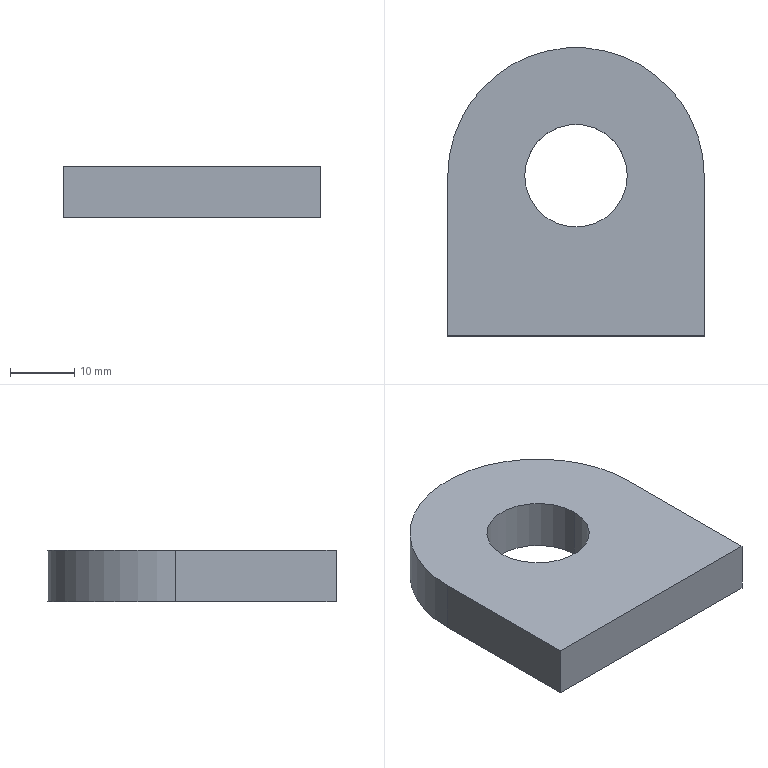Part | SolidWorks | features Extrusion 1 | 1 solid | 8 faces | box 40 x 45 x 8 mm | volume 11418 mm3 | plane 5 | cylinder 3 | commonest cylinder face diameters 16 x2 40 x1
STEP:
#1=CARTESIAN_POINT('',(-8.,0.,8.));
#2=VERTEX_POINT('',#1);
#3=CARTESIAN_POINT('',(8.,0.,8.));
#4=VERTEX_POINT('',#3);
#5=CARTESIAN_POINT('',(0.,0.,8.));
#6=DIRECTION('',(0.,0.,1.));
#7=DIRECTION('',(1.,0.,0.));
#8=AXIS2_PLACEMENT_3D('',#5,#6,#7);
#9=CIRCLE('',#8,8.);
#10=EDGE_CURVE('',#2,#4,#9,.T.);
#11=ORIENTED_EDGE('',*,*,#10,.T.);
#12=CARTESIAN_POINT('',(8.,0.,0.));
#13=VERTEX_POINT('',#12);
#14=CARTESIAN_POINT('',(8.,0.,8.));
#15=DIRECTION('',(0.,0.,-1.));
#16=VECTOR('',#15,1000.);
#17=LINE('',#14,#16);
#18=EDGE_CURVE('',#4,#13,#17,.T.);
#19=ORIENTED_EDGE('',*,*,#18,.T.);
#20=CARTESIAN_POINT('',(-8.,0.,0.));
#21=VERTEX_POINT('',#20);
#22=CARTESIAN_POINT('',(0.,0.,0.));
#23=DIRECTION('',(0.,0.,1.));
#24=DIRECTION('',(1.,0.,0.));
#25=AXIS2_PLACEMENT_3D('',#22,#23,#24);
#26=CIRCLE('',#25,8.);
#27=EDGE_CURVE('',#21,#13,#26,.T.);
#28=ORIENTED_EDGE('',*,*,#27,.F.);
#29=CARTESIAN_POINT('',(-8.,0.,8.));
#30=DIRECTION('',(0.,0.,-1.));
#31=VECTOR('',#30,1000.);
#32=LINE('',#29,#31);
#33=EDGE_CURVE('',#2,#21,#32,.T.);
#34=ORIENTED_EDGE('',*,*,#33,.F.);
#35=EDGE_LOOP('',(#11,#19,#28,#34));
#36=FACE_OUTER_BOUND('',#35,.T.);
#37=CARTESIAN_POINT('',(0.,0.,8.));
#38=DIRECTION('',(0.,0.,-1.));
#39=DIRECTION('',(-1.,0.,0.));
#40=AXIS2_PLACEMENT_3D('',#37,#38,#39);
#41=CYLINDRICAL_SURFACE('',#40,8.);
#42=ADVANCED_FACE('',(#36),#41,.F.);
#43=CARTESIAN_POINT('',(20.,-25.,8.));
#44=VERTEX_POINT('',#43);
#45=CARTESIAN_POINT('',(20.,0.,8.));
#46=VERTEX_POINT('',#45);
#47=CARTESIAN_POINT('',(20.,-25.,8.));
#48=DIRECTION('',(0.,1.,0.));
#49=VECTOR('',#48,1000.);
#50=LINE('',#47,#49);
#51=EDGE_CURVE('',#44,#46,#50,.T.);
#52=ORIENTED_EDGE('',*,*,#51,.T.);
#53=CARTESIAN_POINT('',(-20.,0.,8.));
#54=VERTEX_POINT('',#53);
#55=CARTESIAN_POINT('',(0.,0.,8.));
#56=DIRECTION('',(0.,0.,1.));
#57=DIRECTION('',(1.,0.,0.));
#58=AXIS2_PLACEMENT_3D('',#55,#56,#57);
#59=CIRCLE('',#58,20.);
#60=EDGE_CURVE('',#46,#54,#59,.T.);
#61=ORIENTED_EDGE('',*,*,#60,.T.);
#62=CARTESIAN_POINT('',(-20.,-25.,8.));
#63=VERTEX_POINT('',#62);
#64=CARTESIAN_POINT('',(-20.,0.,8.));
#65=DIRECTION('',(0.,-1.,0.));
#66=VECTOR('',#65,1000.);
#67=LINE('',#64,#66);
#68=EDGE_CURVE('',#54,#63,#67,.T.);
#69=ORIENTED_EDGE('',*,*,#68,.T.);
#70=CARTESIAN_POINT('',(-20.,-25.,8.));
#71=DIRECTION('',(1.,0.,0.));
#72=VECTOR('',#71,1000.);
#73=LINE('',#70,#72);
#74=EDGE_CURVE('',#63,#44,#73,.T.);
#75=ORIENTED_EDGE('',*,*,#74,.T.);
#76=EDGE_LOOP('',(#52,#61,#69,#75));
#77=FACE_OUTER_BOUND('',#76,.T.);
#78=ORIENTED_EDGE('',*,*,#10,.F.);
#79=CARTESIAN_POINT('',(0.,0.,8.));
#80=DIRECTION('',(0.,0.,1.));
#81=DIRECTION('',(1.,0.,0.));
#82=AXIS2_PLACEMENT_3D('',#79,#80,#81);
#83=CIRCLE('',#82,8.);
#84=EDGE_CURVE('',#4,#2,#83,.T.);
#85=ORIENTED_EDGE('',*,*,#84,.F.);
#86=EDGE_LOOP('',(#78,#85));
#87=FACE_BOUND('',#86,.T.);
#88=CARTESIAN_POINT('',(0.,0.,8.));
#89=DIRECTION('',(0.,0.,1.));
#90=DIRECTION('',(1.,0.,0.));
#91=AXIS2_PLACEMENT_3D('',#88,#89,#90);
#92=PLANE('',#91);
#93=ADVANCED_FACE('',(#77,#87),#92,.T.);
#94=CARTESIAN_POINT('',(20.,-25.,0.));
#95=VERTEX_POINT('',#94);
#96=CARTESIAN_POINT('',(20.,0.,0.));
#97=VERTEX_POINT('',#96);
#98=CARTESIAN_POINT('',(20.,-25.,0.));
#99=DIRECTION('',(0.,1.,0.));
#100=VECTOR('',#99,1000.);
#101=LINE('',#98,#100);
#102=EDGE_CURVE('',#95,#97,#101,.T.);
#103=ORIENTED_EDGE('',*,*,#102,.F.);
#104=CARTESIAN_POINT('',(-20.,-25.,0.));
#105=VERTEX_POINT('',#104);
#106=CARTESIAN_POINT('',(-20.,-25.,0.));
#107=DIRECTION('',(1.,0.,0.));
#108=VECTOR('',#107,1000.);
#109=LINE('',#106,#108);
#110=EDGE_CURVE('',#105,#95,#109,.T.);
#111=ORIENTED_EDGE('',*,*,#110,.F.);
#112=CARTESIAN_POINT('',(-20.,0.,0.));
#113=VERTEX_POINT('',#112);
#114=CARTESIAN_POINT('',(-20.,0.,0.));
#115=DIRECTION('',(0.,-1.,0.));
#116=VECTOR('',#115,1000.);
#117=LINE('',#114,#116);
#118=EDGE_CURVE('',#113,#105,#117,.T.);
#119=ORIENTED_EDGE('',*,*,#118,.F.);
#120=CARTESIAN_POINT('',(0.,0.,0.));
#121=DIRECTION('',(0.,0.,1.));
#122=DIRECTION('',(1.,0.,0.));
#123=AXIS2_PLACEMENT_3D('',#120,#121,#122);
#124=CIRCLE('',#123,20.);
#125=EDGE_CURVE('',#97,#113,#124,.T.);
#126=ORIENTED_EDGE('',*,*,#125,.F.);
#127=EDGE_LOOP('',(#103,#111,#119,#126));
#128=FACE_OUTER_BOUND('',#127,.T.);
#129=ORIENTED_EDGE('',*,*,#27,.T.);
#130=CARTESIAN_POINT('',(0.,0.,0.));
#131=DIRECTION('',(0.,0.,1.));
#132=DIRECTION('',(1.,0.,0.));
#133=AXIS2_PLACEMENT_3D('',#130,#131,#132);
#134=CIRCLE('',#133,8.);
#135=EDGE_CURVE('',#13,#21,#134,.T.);
#136=ORIENTED_EDGE('',*,*,#135,.T.);
#137=EDGE_LOOP('',(#129,#136));
#138=FACE_BOUND('',#137,.T.);
#139=CARTESIAN_POINT('',(0.,0.,0.));
#140=DIRECTION('',(0.,0.,1.));
#141=DIRECTION('',(1.,0.,0.));
#142=AXIS2_PLACEMENT_3D('',#139,#140,#141);
#143=PLANE('',#142);
#144=ADVANCED_FACE('',(#128,#138),#143,.F.);
#145=ORIENTED_EDGE('',*,*,#102,.T.);
#146=CARTESIAN_POINT('',(20.,0.,8.));
#147=DIRECTION('',(0.,0.,-1.));
#148=VECTOR('',#147,1000.);
#149=LINE('',#146,#148);
#150=EDGE_CURVE('',#46,#97,#149,.T.);
#151=ORIENTED_EDGE('',*,*,#150,.F.);
#152=ORIENTED_EDGE('',*,*,#51,.F.);
#153=CARTESIAN_POINT('',(20.,-25.,8.));
#154=DIRECTION('',(0.,0.,-1.));
#155=VECTOR('',#154,1000.);
#156=LINE('',#153,#155);
#157=EDGE_CURVE('',#44,#95,#156,.T.);
#158=ORIENTED_EDGE('',*,*,#157,.T.);
#159=EDGE_LOOP('',(#145,#151,#152,#158));
#160=FACE_OUTER_BOUND('',#159,.T.);
#161=CARTESIAN_POINT('',(20.,-25.,8.));
#162=DIRECTION('',(-1.,0.,0.));
#163=DIRECTION('',(0.,-1.,0.));
#164=AXIS2_PLACEMENT_3D('',#161,#162,#163);
#165=PLANE('',#164);
#166=ADVANCED_FACE('',(#160),#165,.F.);
#167=ORIENTED_EDGE('',*,*,#125,.T.);
#168=CARTESIAN_POINT('',(-20.,0.,8.));
#169=DIRECTION('',(0.,0.,-1.));
#170=VECTOR('',#169,1000.);
#171=LINE('',#168,#170);
#172=EDGE_CURVE('',#54,#113,#171,.T.);
#173=ORIENTED_EDGE('',*,*,#172,.F.);
#174=ORIENTED_EDGE('',*,*,#60,.F.);
#175=ORIENTED_EDGE('',*,*,#150,.T.);
#176=EDGE_LOOP('',(#167,#173,#174,#175));
#177=FACE_OUTER_BOUND('',#176,.T.);
#178=CARTESIAN_POINT('',(0.,0.,8.));
#179=DIRECTION('',(0.,0.,-1.));
#180=DIRECTION('',(-1.,0.,0.));
#181=AXIS2_PLACEMENT_3D('',#178,#179,#180);
#182=CYLINDRICAL_SURFACE('',#181,20.);
#183=ADVANCED_FACE('',(#177),#182,.T.);
#184=ORIENTED_EDGE('',*,*,#118,.T.);
#185=CARTESIAN_POINT('',(-20.,-25.,8.));
#186=DIRECTION('',(0.,0.,-1.));
#187=VECTOR('',#186,1000.);
#188=LINE('',#185,#187);
#189=EDGE_CURVE('',#63,#105,#188,.T.);
#190=ORIENTED_EDGE('',*,*,#189,.F.);
#191=ORIENTED_EDGE('',*,*,#68,.F.);
#192=ORIENTED_EDGE('',*,*,#172,.T.);
#193=EDGE_LOOP('',(#184,#190,#191,#192));
#194=FACE_OUTER_BOUND('',#193,.T.);
#195=CARTESIAN_POINT('',(-20.,0.,8.));
#196=DIRECTION('',(1.,0.,0.));
#197=DIRECTION('',(0.,1.,0.));
#198=AXIS2_PLACEMENT_3D('',#195,#196,#197);
#199=PLANE('',#198);
#200=ADVANCED_FACE('',(#194),#199,.F.);
#201=ORIENTED_EDGE('',*,*,#110,.T.);
#202=ORIENTED_EDGE('',*,*,#157,.F.);
#203=ORIENTED_EDGE('',*,*,#74,.F.);
#204=ORIENTED_EDGE('',*,*,#189,.T.);
#205=EDGE_LOOP('',(#201,#202,#203,#204));
#206=FACE_OUTER_BOUND('',#205,.T.);
#207=CARTESIAN_POINT('',(-20.,-25.,8.));
#208=DIRECTION('',(0.,1.,0.));
#209=DIRECTION('',(0.,0.,1.));
#210=AXIS2_PLACEMENT_3D('',#207,#208,#209);
#211=PLANE('',#210);
#212=ADVANCED_FACE('',(#206),#211,.F.);
#213=ORIENTED_EDGE('',*,*,#18,.F.);
#214=ORIENTED_EDGE('',*,*,#84,.T.);
#215=ORIENTED_EDGE('',*,*,#33,.T.);
#216=ORIENTED_EDGE('',*,*,#135,.F.);
#217=EDGE_LOOP('',(#213,#214,#215,#216));
#218=FACE_OUTER_BOUND('',#217,.T.);
#219=CARTESIAN_POINT('',(0.,0.,8.));
#220=DIRECTION('',(0.,0.,-1.));
#221=DIRECTION('',(-1.,0.,0.));
#222=AXIS2_PLACEMENT_3D('',#219,#220,#221);
#223=CYLINDRICAL_SURFACE('',#222,8.);
#224=ADVANCED_FACE('',(#218),#223,.F.);
#225=CLOSED_SHELL('',(#42,#93,#144,#166,#183,#200,#212,#224));
#226=MANIFOLD_SOLID_BREP('',#225);
#227=CARTESIAN_POINT('',(0.,0.,0.));
#228=DIRECTION('',(0.,0.,1.));
#229=DIRECTION('',(1.,0.,0.));
#230=AXIS2_PLACEMENT_3D('',#227,#228,#229);
#231=(LENGTH_UNIT()NAMED_UNIT(*)SI_UNIT(.MILLI.,.METRE.));
#232=UNCERTAINTY_MEASURE_WITH_UNIT(LENGTH_MEASURE(0.00001),#231,'','');
#233=(NAMED_UNIT(*)PLANE_ANGLE_UNIT()SI_UNIT($,.RADIAN.));
#234=(NAMED_UNIT(*)SI_UNIT($,.STERADIAN.)SOLID_ANGLE_UNIT());
#235=(GEOMETRIC_REPRESENTATION_CONTEXT(3)GLOBAL_UNCERTAINTY_ASSIGNED_CONTEXT((#232))GLOBAL_UNIT_ASSIGNED_CONTEXT((#231,#233,#234))REPRESENTATION_CONTEXT('',''));
#236=ADVANCED_BREP_SHAPE_REPRESENTATION('',(#226,#230),#235);